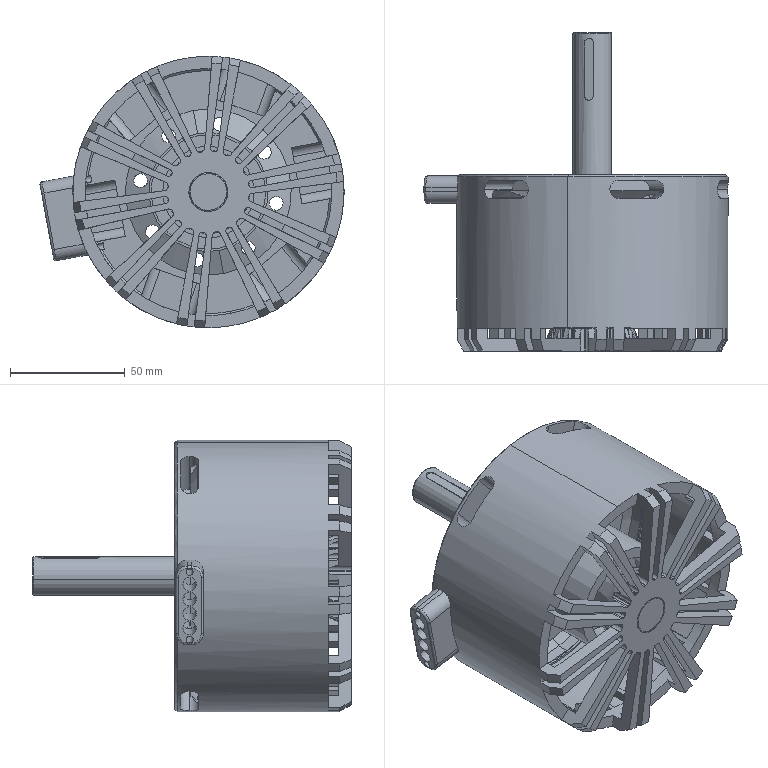Part | SolidWorks | features BaseBody 1 | 1 solid | 481 faces | box 132.717 x 139 x 118.4 mm | volume 257546 mm3 | plane 267 | cylinder 173 | cone 33 | torus 8 | commonest cylinder face diameters 3 x28 3.6 x26 6 x24 7.98 x24 35.485 x21 17 x8